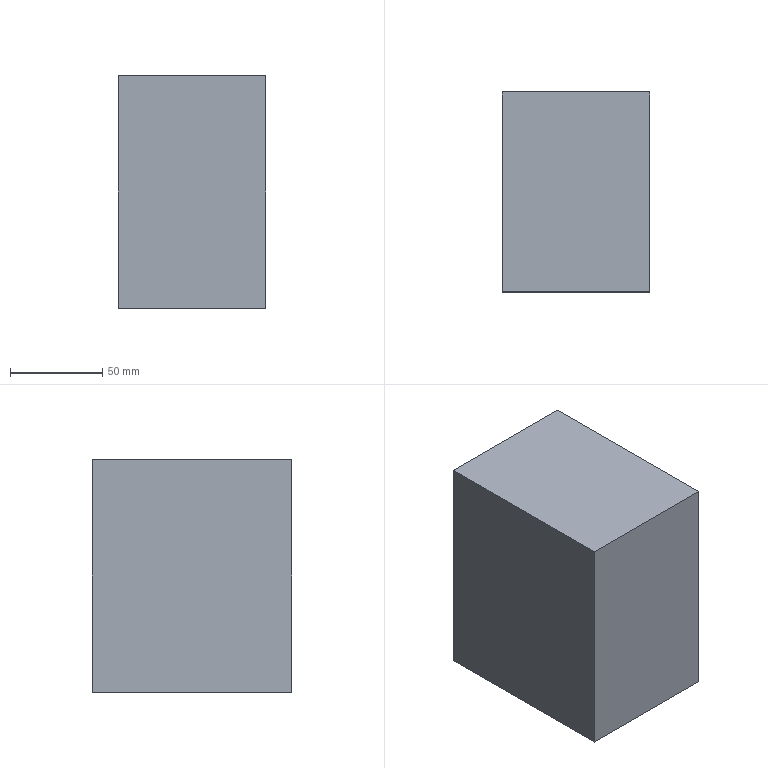Part | SolidWorks | features Extrusion 1, HoleWzd 1 | 1 solid | 14 faces | box 80 x 108 x 126 mm | volume 954806 mm3 | plane 6 | cylinder 4 | cone 4 | commonest cylinder face diameters 32 x4
STEP:
#1=CARTESIAN_POINT('',(0.,-26.,-50.));
#2=VERTEX_POINT('',#1);
#3=CARTESIAN_POINT('',(0.,-26.,-18.));
#4=VERTEX_POINT('',#3);
#5=CARTESIAN_POINT('',(0.,-26.,-34.));
#6=DIRECTION('',(0.,1.,0.));
#7=DIRECTION('',(0.,0.,1.));
#8=AXIS2_PLACEMENT_3D('',#5,#6,#7);
#9=CIRCLE('',#8,16.);
#10=EDGE_CURVE('',#2,#4,#9,.T.);
#11=ORIENTED_EDGE('',*,*,#10,.F.);
#12=CARTESIAN_POINT('',(0.,54.,-50.));
#13=VERTEX_POINT('',#12);
#14=CARTESIAN_POINT('',(0.,54.,-50.));
#15=DIRECTION('',(0.,1.,0.));
#16=VECTOR('',#15,1000.);
#17=LINE('',#14,#16);
#18=EDGE_CURVE('',#2,#13,#17,.T.);
#19=ORIENTED_EDGE('',*,*,#18,.T.);
#20=CARTESIAN_POINT('',(0.,54.,-18.));
#21=VERTEX_POINT('',#20);
#22=CARTESIAN_POINT('',(0.,54.,-34.));
#23=DIRECTION('',(0.,1.,0.));
#24=DIRECTION('',(0.,0.,1.));
#25=AXIS2_PLACEMENT_3D('',#22,#23,#24);
#26=CIRCLE('',#25,16.);
#27=EDGE_CURVE('',#13,#21,#26,.T.);
#28=ORIENTED_EDGE('',*,*,#27,.T.);
#29=CARTESIAN_POINT('',(0.,54.,-18.));
#30=DIRECTION('',(0.,1.,0.));
#31=VECTOR('',#30,1000.);
#32=LINE('',#29,#31);
#33=EDGE_CURVE('',#4,#21,#32,.T.);
#34=ORIENTED_EDGE('',*,*,#33,.F.);
#35=EDGE_LOOP('',(#11,#19,#28,#34));
#36=FACE_OUTER_BOUND('',#35,.T.);
#37=CARTESIAN_POINT('',(0.,54.,-34.));
#38=DIRECTION('',(0.,1.,0.));
#39=DIRECTION('',(0.,0.,1.));
#40=AXIS2_PLACEMENT_3D('',#37,#38,#39);
#41=CYLINDRICAL_SURFACE('',#40,16.);
#42=ADVANCED_FACE('',(#36),#41,.F.);
#43=CARTESIAN_POINT('',(0.,-35.614,-34.));
#44=VERTEX_POINT('',#43);
#45=CARTESIAN_POINT('',(0.,-26.,-18.));
#46=DIRECTION('',(0.,0.515,0.8572));
#47=VECTOR('',#46,1000.);
#48=LINE('',#45,#47);
#49=EDGE_CURVE('',#44,#4,#48,.T.);
#50=ORIENTED_EDGE('',*,*,#49,.F.);
#51=CARTESIAN_POINT('',(0.,-26.,-50.));
#52=DIRECTION('',(0.,0.515,-0.8572));
#53=VECTOR('',#52,1000.);
#54=LINE('',#51,#53);
#55=EDGE_CURVE('',#44,#2,#54,.T.);
#56=ORIENTED_EDGE('',*,*,#55,.T.);
#57=ORIENTED_EDGE('',*,*,#10,.T.);
#58=EDGE_LOOP('',(#50,#56,#57));
#59=FACE_OUTER_BOUND('',#58,.T.);
#60=CARTESIAN_POINT('',(0.,-26.,-34.));
#61=DIRECTION('',(0.,1.,0.));
#62=DIRECTION('',(0.,0.,1.));
#63=AXIS2_PLACEMENT_3D('',#60,#61,#62);
#64=CONICAL_SURFACE('',#63,16.,1.03);
#65=ADVANCED_FACE('',(#59),#64,.F.);
#66=CARTESIAN_POINT('',(0.,-26.,18.));
#67=VERTEX_POINT('',#66);
#68=CARTESIAN_POINT('',(0.,-26.,50.));
#69=VERTEX_POINT('',#68);
#70=CARTESIAN_POINT('',(0.,-26.,34.));
#71=DIRECTION('',(0.,1.,0.));
#72=DIRECTION('',(0.,0.,1.));
#73=AXIS2_PLACEMENT_3D('',#70,#71,#72);
#74=CIRCLE('',#73,16.);
#75=EDGE_CURVE('',#67,#69,#74,.T.);
#76=ORIENTED_EDGE('',*,*,#75,.F.);
#77=CARTESIAN_POINT('',(0.,54.,18.));
#78=VERTEX_POINT('',#77);
#79=CARTESIAN_POINT('',(0.,54.,18.));
#80=DIRECTION('',(0.,1.,0.));
#81=VECTOR('',#80,1000.);
#82=LINE('',#79,#81);
#83=EDGE_CURVE('',#67,#78,#82,.T.);
#84=ORIENTED_EDGE('',*,*,#83,.T.);
#85=CARTESIAN_POINT('',(0.,54.,50.));
#86=VERTEX_POINT('',#85);
#87=CARTESIAN_POINT('',(0.,54.,34.));
#88=DIRECTION('',(0.,1.,0.));
#89=DIRECTION('',(0.,0.,1.));
#90=AXIS2_PLACEMENT_3D('',#87,#88,#89);
#91=CIRCLE('',#90,16.);
#92=EDGE_CURVE('',#78,#86,#91,.T.);
#93=ORIENTED_EDGE('',*,*,#92,.T.);
#94=CARTESIAN_POINT('',(0.,54.,50.));
#95=DIRECTION('',(0.,1.,0.));
#96=VECTOR('',#95,1000.);
#97=LINE('',#94,#96);
#98=EDGE_CURVE('',#69,#86,#97,.T.);
#99=ORIENTED_EDGE('',*,*,#98,.F.);
#100=EDGE_LOOP('',(#76,#84,#93,#99));
#101=FACE_OUTER_BOUND('',#100,.T.);
#102=CARTESIAN_POINT('',(0.,54.,34.));
#103=DIRECTION('',(0.,1.,0.));
#104=DIRECTION('',(0.,0.,1.));
#105=AXIS2_PLACEMENT_3D('',#102,#103,#104);
#106=CYLINDRICAL_SURFACE('',#105,16.);
#107=ADVANCED_FACE('',(#101),#106,.F.);
#108=CARTESIAN_POINT('',(0.,-35.614,34.));
#109=VERTEX_POINT('',#108);
#110=CARTESIAN_POINT('',(0.,-26.,50.));
#111=DIRECTION('',(0.,0.515,0.8572));
#112=VECTOR('',#111,1000.);
#113=LINE('',#110,#112);
#114=EDGE_CURVE('',#109,#69,#113,.T.);
#115=ORIENTED_EDGE('',*,*,#114,.F.);
#116=CARTESIAN_POINT('',(0.,-26.,18.));
#117=DIRECTION('',(0.,0.515,-0.8572));
#118=VECTOR('',#117,1000.);
#119=LINE('',#116,#118);
#120=EDGE_CURVE('',#109,#67,#119,.T.);
#121=ORIENTED_EDGE('',*,*,#120,.T.);
#122=ORIENTED_EDGE('',*,*,#75,.T.);
#123=EDGE_LOOP('',(#115,#121,#122));
#124=FACE_OUTER_BOUND('',#123,.T.);
#125=CARTESIAN_POINT('',(0.,-26.,34.));
#126=DIRECTION('',(0.,1.,0.));
#127=DIRECTION('',(0.,0.,1.));
#128=AXIS2_PLACEMENT_3D('',#125,#126,#127);
#129=CONICAL_SURFACE('',#128,16.,1.03);
#130=ADVANCED_FACE('',(#124),#129,.F.);
#131=CARTESIAN_POINT('',(-40.,-54.,-63.));
#132=VERTEX_POINT('',#131);
#133=CARTESIAN_POINT('',(-40.,-54.,63.));
#134=VERTEX_POINT('',#133);
#135=CARTESIAN_POINT('',(-40.,-54.,-63.));
#136=DIRECTION('',(0.,0.,1.));
#137=VECTOR('',#136,1000.);
#138=LINE('',#135,#137);
#139=EDGE_CURVE('',#132,#134,#138,.T.);
#140=ORIENTED_EDGE('',*,*,#139,.T.);
#141=CARTESIAN_POINT('',(-40.,54.,63.));
#142=VERTEX_POINT('',#141);
#143=CARTESIAN_POINT('',(-40.,54.,63.));
#144=DIRECTION('',(0.,-1.,0.));
#145=VECTOR('',#144,1000.);
#146=LINE('',#143,#145);
#147=EDGE_CURVE('',#142,#134,#146,.T.);
#148=ORIENTED_EDGE('',*,*,#147,.F.);
#149=CARTESIAN_POINT('',(-40.,54.,-63.));
#150=VERTEX_POINT('',#149);
#151=CARTESIAN_POINT('',(-40.,54.,-63.));
#152=DIRECTION('',(0.,0.,1.));
#153=VECTOR('',#152,1000.);
#154=LINE('',#151,#153);
#155=EDGE_CURVE('',#150,#142,#154,.T.);
#156=ORIENTED_EDGE('',*,*,#155,.F.);
#157=CARTESIAN_POINT('',(-40.,54.,-63.));
#158=DIRECTION('',(0.,-1.,0.));
#159=VECTOR('',#158,1000.);
#160=LINE('',#157,#159);
#161=EDGE_CURVE('',#150,#132,#160,.T.);
#162=ORIENTED_EDGE('',*,*,#161,.T.);
#163=EDGE_LOOP('',(#140,#148,#156,#162));
#164=FACE_OUTER_BOUND('',#163,.T.);
#165=CARTESIAN_POINT('',(-40.,54.,-63.));
#166=DIRECTION('',(1.,0.,0.));
#167=DIRECTION('',(0.,0.,-1.));
#168=AXIS2_PLACEMENT_3D('',#165,#166,#167);
#169=PLANE('',#168);
#170=ADVANCED_FACE('',(#164),#169,.F.);
#171=CARTESIAN_POINT('',(40.,-54.,63.));
#172=VERTEX_POINT('',#171);
#173=CARTESIAN_POINT('',(-40.,-54.,63.));
#174=DIRECTION('',(1.,0.,0.));
#175=VECTOR('',#174,1000.);
#176=LINE('',#173,#175);
#177=EDGE_CURVE('',#134,#172,#176,.T.);
#178=ORIENTED_EDGE('',*,*,#177,.T.);
#179=CARTESIAN_POINT('',(40.,54.,63.));
#180=VERTEX_POINT('',#179);
#181=CARTESIAN_POINT('',(40.,54.,63.));
#182=DIRECTION('',(0.,-1.,0.));
#183=VECTOR('',#182,1000.);
#184=LINE('',#181,#183);
#185=EDGE_CURVE('',#180,#172,#184,.T.);
#186=ORIENTED_EDGE('',*,*,#185,.F.);
#187=CARTESIAN_POINT('',(-40.,54.,63.));
#188=DIRECTION('',(1.,0.,0.));
#189=VECTOR('',#188,1000.);
#190=LINE('',#187,#189);
#191=EDGE_CURVE('',#142,#180,#190,.T.);
#192=ORIENTED_EDGE('',*,*,#191,.F.);
#193=ORIENTED_EDGE('',*,*,#147,.T.);
#194=EDGE_LOOP('',(#178,#186,#192,#193));
#195=FACE_OUTER_BOUND('',#194,.T.);
#196=CARTESIAN_POINT('',(-40.,54.,63.));
#197=DIRECTION('',(0.,0.,-1.));
#198=DIRECTION('',(-1.,0.,0.));
#199=AXIS2_PLACEMENT_3D('',#196,#197,#198);
#200=PLANE('',#199);
#201=ADVANCED_FACE('',(#195),#200,.F.);
#202=CARTESIAN_POINT('',(40.,-54.,-63.));
#203=VERTEX_POINT('',#202);
#204=CARTESIAN_POINT('',(40.,-54.,-63.));
#205=DIRECTION('',(0.,0.,-1.));
#206=VECTOR('',#205,1000.);
#207=LINE('',#204,#206);
#208=EDGE_CURVE('',#172,#203,#207,.T.);
#209=ORIENTED_EDGE('',*,*,#208,.T.);
#210=CARTESIAN_POINT('',(40.,54.,-63.));
#211=VERTEX_POINT('',#210);
#212=CARTESIAN_POINT('',(40.,54.,-63.));
#213=DIRECTION('',(0.,-1.,0.));
#214=VECTOR('',#213,1000.);
#215=LINE('',#212,#214);
#216=EDGE_CURVE('',#211,#203,#215,.T.);
#217=ORIENTED_EDGE('',*,*,#216,.F.);
#218=CARTESIAN_POINT('',(40.,54.,-63.));
#219=DIRECTION('',(0.,0.,-1.));
#220=VECTOR('',#219,1000.);
#221=LINE('',#218,#220);
#222=EDGE_CURVE('',#180,#211,#221,.T.);
#223=ORIENTED_EDGE('',*,*,#222,.F.);
#224=ORIENTED_EDGE('',*,*,#185,.T.);
#225=EDGE_LOOP('',(#209,#217,#223,#224));
#226=FACE_OUTER_BOUND('',#225,.T.);
#227=CARTESIAN_POINT('',(40.,54.,-63.));
#228=DIRECTION('',(-1.,0.,0.));
#229=DIRECTION('',(0.,0.,1.));
#230=AXIS2_PLACEMENT_3D('',#227,#228,#229);
#231=PLANE('',#230);
#232=ADVANCED_FACE('',(#226),#231,.F.);
#233=CARTESIAN_POINT('',(-40.,-54.,-63.));
#234=DIRECTION('',(-1.,0.,0.));
#235=VECTOR('',#234,1000.);
#236=LINE('',#233,#235);
#237=EDGE_CURVE('',#203,#132,#236,.T.);
#238=ORIENTED_EDGE('',*,*,#237,.T.);
#239=ORIENTED_EDGE('',*,*,#161,.F.);
#240=CARTESIAN_POINT('',(-40.,54.,-63.));
#241=DIRECTION('',(-1.,0.,0.));
#242=VECTOR('',#241,1000.);
#243=LINE('',#240,#242);
#244=EDGE_CURVE('',#211,#150,#243,.T.);
#245=ORIENTED_EDGE('',*,*,#244,.F.);
#246=ORIENTED_EDGE('',*,*,#216,.T.);
#247=EDGE_LOOP('',(#238,#239,#245,#246));
#248=FACE_OUTER_BOUND('',#247,.T.);
#249=CARTESIAN_POINT('',(-40.,54.,-63.));
#250=DIRECTION('',(0.,0.,1.));
#251=DIRECTION('',(1.,0.,0.));
#252=AXIS2_PLACEMENT_3D('',#249,#250,#251);
#253=PLANE('',#252);
#254=ADVANCED_FACE('',(#248),#253,.F.);
#255=CARTESIAN_POINT('',(0.,54.,-34.));
#256=DIRECTION('',(0.,1.,0.));
#257=DIRECTION('',(0.,0.,1.));
#258=AXIS2_PLACEMENT_3D('',#255,#256,#257);
#259=CIRCLE('',#258,16.);
#260=EDGE_CURVE('',#21,#13,#259,.T.);
#261=ORIENTED_EDGE('',*,*,#260,.F.);
#262=ORIENTED_EDGE('',*,*,#27,.F.);
#263=EDGE_LOOP('',(#261,#262));
#264=FACE_BOUND('',#263,.T.);
#265=CARTESIAN_POINT('',(0.,54.,34.));
#266=DIRECTION('',(0.,1.,0.));
#267=DIRECTION('',(0.,0.,1.));
#268=AXIS2_PLACEMENT_3D('',#265,#266,#267);
#269=CIRCLE('',#268,16.);
#270=EDGE_CURVE('',#86,#78,#269,.T.);
#271=ORIENTED_EDGE('',*,*,#270,.F.);
#272=ORIENTED_EDGE('',*,*,#92,.F.);
#273=EDGE_LOOP('',(#271,#272));
#274=FACE_BOUND('',#273,.T.);
#275=ORIENTED_EDGE('',*,*,#155,.T.);
#276=ORIENTED_EDGE('',*,*,#191,.T.);
#277=ORIENTED_EDGE('',*,*,#222,.T.);
#278=ORIENTED_EDGE('',*,*,#244,.T.);
#279=EDGE_LOOP('',(#275,#276,#277,#278));
#280=FACE_OUTER_BOUND('',#279,.T.);
#281=CARTESIAN_POINT('',(0.,54.,0.));
#282=DIRECTION('',(0.,1.,0.));
#283=DIRECTION('',(0.,0.,1.));
#284=AXIS2_PLACEMENT_3D('',#281,#282,#283);
#285=PLANE('',#284);
#286=ADVANCED_FACE('',(#264,#274,#280),#285,.T.);
#287=ORIENTED_EDGE('',*,*,#139,.F.);
#288=ORIENTED_EDGE('',*,*,#237,.F.);
#289=ORIENTED_EDGE('',*,*,#208,.F.);
#290=ORIENTED_EDGE('',*,*,#177,.F.);
#291=EDGE_LOOP('',(#287,#288,#289,#290));
#292=FACE_OUTER_BOUND('',#291,.T.);
#293=CARTESIAN_POINT('',(0.,-54.,0.));
#294=DIRECTION('',(0.,1.,0.));
#295=DIRECTION('',(0.,0.,1.));
#296=AXIS2_PLACEMENT_3D('',#293,#294,#295);
#297=PLANE('',#296);
#298=ADVANCED_FACE('',(#292),#297,.F.);
#299=ORIENTED_EDGE('',*,*,#120,.F.);
#300=ORIENTED_EDGE('',*,*,#114,.T.);
#301=CARTESIAN_POINT('',(0.,-26.,34.));
#302=DIRECTION('',(0.,1.,0.));
#303=DIRECTION('',(0.,0.,1.));
#304=AXIS2_PLACEMENT_3D('',#301,#302,#303);
#305=CIRCLE('',#304,16.);
#306=EDGE_CURVE('',#69,#67,#305,.T.);
#307=ORIENTED_EDGE('',*,*,#306,.T.);
#308=EDGE_LOOP('',(#299,#300,#307));
#309=FACE_OUTER_BOUND('',#308,.T.);
#310=CARTESIAN_POINT('',(0.,-26.,34.));
#311=DIRECTION('',(0.,1.,0.));
#312=DIRECTION('',(0.,0.,1.));
#313=AXIS2_PLACEMENT_3D('',#310,#311,#312);
#314=CONICAL_SURFACE('',#313,16.,1.03);
#315=ADVANCED_FACE('',(#309),#314,.F.);
#316=ORIENTED_EDGE('',*,*,#83,.F.);
#317=ORIENTED_EDGE('',*,*,#306,.F.);
#318=ORIENTED_EDGE('',*,*,#98,.T.);
#319=ORIENTED_EDGE('',*,*,#270,.T.);
#320=EDGE_LOOP('',(#316,#317,#318,#319));
#321=FACE_OUTER_BOUND('',#320,.T.);
#322=CARTESIAN_POINT('',(0.,54.,34.));
#323=DIRECTION('',(0.,1.,0.));
#324=DIRECTION('',(0.,0.,1.));
#325=AXIS2_PLACEMENT_3D('',#322,#323,#324);
#326=CYLINDRICAL_SURFACE('',#325,16.);
#327=ADVANCED_FACE('',(#321),#326,.F.);
#328=ORIENTED_EDGE('',*,*,#55,.F.);
#329=ORIENTED_EDGE('',*,*,#49,.T.);
#330=CARTESIAN_POINT('',(0.,-26.,-34.));
#331=DIRECTION('',(0.,1.,0.));
#332=DIRECTION('',(0.,0.,1.));
#333=AXIS2_PLACEMENT_3D('',#330,#331,#332);
#334=CIRCLE('',#333,16.);
#335=EDGE_CURVE('',#4,#2,#334,.T.);
#336=ORIENTED_EDGE('',*,*,#335,.T.);
#337=EDGE_LOOP('',(#328,#329,#336));
#338=FACE_OUTER_BOUND('',#337,.T.);
#339=CARTESIAN_POINT('',(0.,-26.,-34.));
#340=DIRECTION('',(0.,1.,0.));
#341=DIRECTION('',(0.,0.,1.));
#342=AXIS2_PLACEMENT_3D('',#339,#340,#341);
#343=CONICAL_SURFACE('',#342,16.,1.03);
#344=ADVANCED_FACE('',(#338),#343,.F.);
#345=ORIENTED_EDGE('',*,*,#18,.F.);
#346=ORIENTED_EDGE('',*,*,#335,.F.);
#347=ORIENTED_EDGE('',*,*,#33,.T.);
#348=ORIENTED_EDGE('',*,*,#260,.T.);
#349=EDGE_LOOP('',(#345,#346,#347,#348));
#350=FACE_OUTER_BOUND('',#349,.T.);
#351=CARTESIAN_POINT('',(0.,54.,-34.));
#352=DIRECTION('',(0.,1.,0.));
#353=DIRECTION('',(0.,0.,1.));
#354=AXIS2_PLACEMENT_3D('',#351,#352,#353);
#355=CYLINDRICAL_SURFACE('',#354,16.);
#356=ADVANCED_FACE('',(#350),#355,.F.);
#357=CLOSED_SHELL('',(#42,#65,#107,#130,#170,#201,#232,#254,#286,#298,#315,#327,#344,#356));
#358=MANIFOLD_SOLID_BREP('',#357);
#359=CARTESIAN_POINT('',(0.,0.,0.));
#360=DIRECTION('',(0.,0.,1.));
#361=DIRECTION('',(1.,0.,0.));
#362=AXIS2_PLACEMENT_3D('',#359,#360,#361);
#363=(LENGTH_UNIT()NAMED_UNIT(*)SI_UNIT(.MILLI.,.METRE.));
#364=UNCERTAINTY_MEASURE_WITH_UNIT(LENGTH_MEASURE(0.00001),#363,'','');
#365=(NAMED_UNIT(*)PLANE_ANGLE_UNIT()SI_UNIT($,.RADIAN.));
#366=(NAMED_UNIT(*)SI_UNIT($,.STERADIAN.)SOLID_ANGLE_UNIT());
#367=(GEOMETRIC_REPRESENTATION_CONTEXT(3)GLOBAL_UNCERTAINTY_ASSIGNED_CONTEXT((#364))GLOBAL_UNIT_ASSIGNED_CONTEXT((#363,#365,#366))REPRESENTATION_CONTEXT('',''));
#368=ADVANCED_BREP_SHAPE_REPRESENTATION('',(#358,#362),#367);